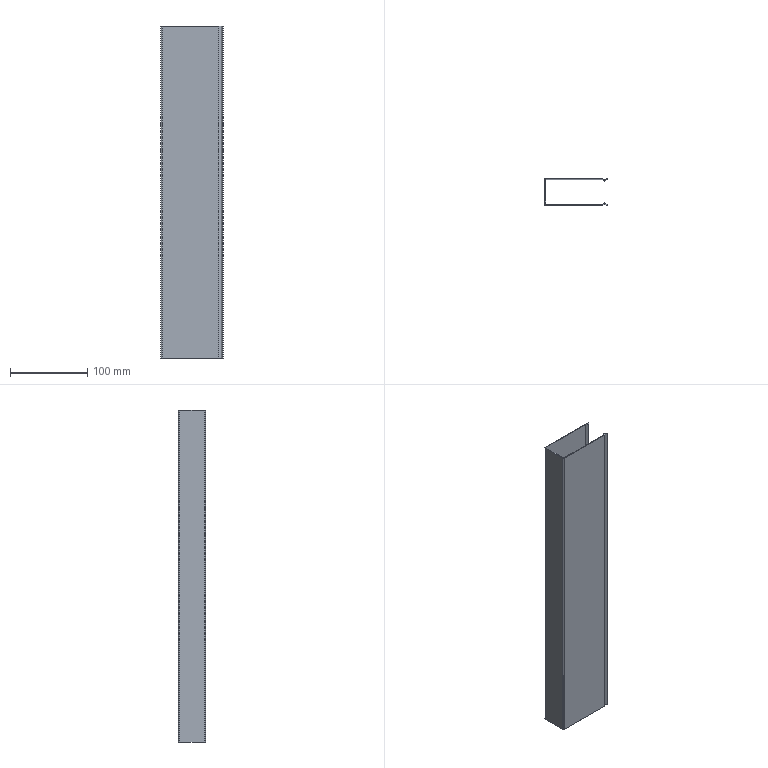Part | STEP file | Cable trough 35_L430 | 1 solid | 22 faces | box 80.625 x 35 x 430 mm | volume 84214 mm3 | plane 18 | cylinder 4 | commonest cylinder face diameters 1 x2 3 x2